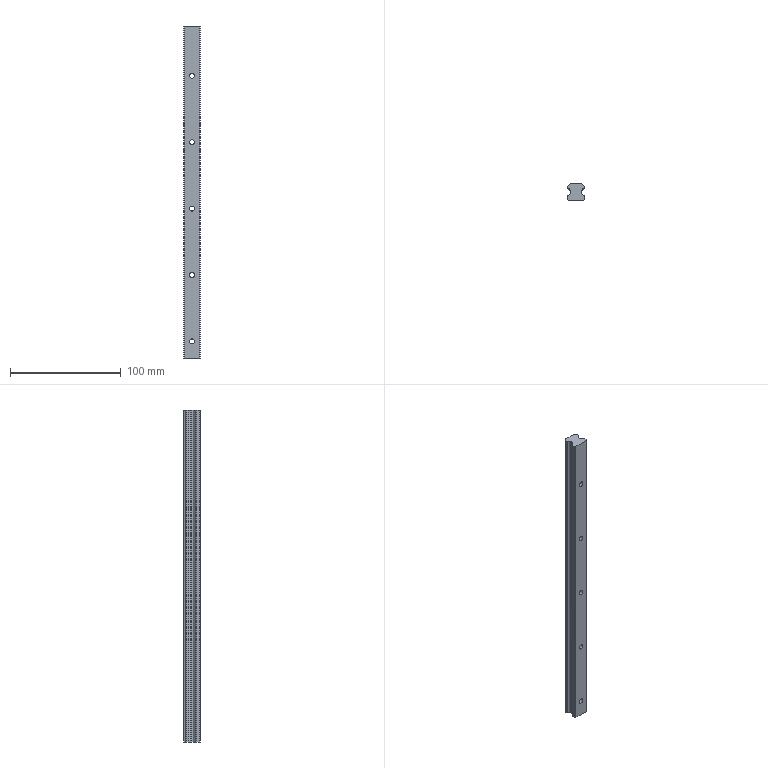Part | STEP file | 1 solid | 61 faces | box 15 x 15 x 300 mm | volume 55463 mm3 | cylinder 34 | plane 27 | commonest cylinder face diameters 4.5 x10 7.5 x10 0.8 x8 3.24 x4 2 x2